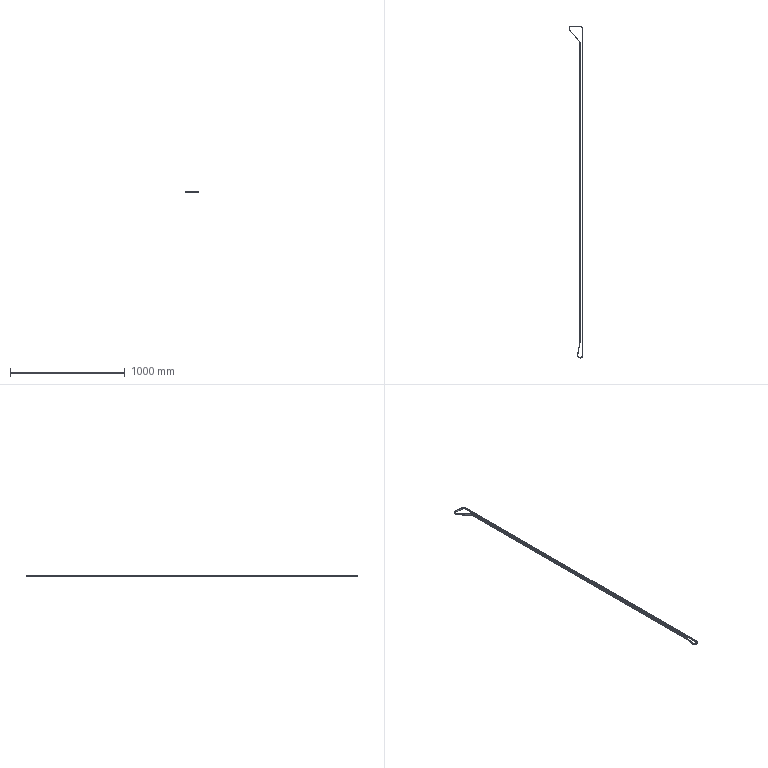Part | SolidWorks | features BaseBody 1 | 1 solid | 26 faces | box 118.8 x 2900 x 15 mm | volume 178480 mm3 | cylinder 14 | plane 12 | commonest cylinder face diameters 41.8 x5 45.8 x5 23 x2 27 x2
STEP:
#1=CARTESIAN_POINT('',(-71.857,624.869,16.));
#2=VERTEX_POINT('',#1);
#3=CARTESIAN_POINT('',(-93.9,604.,16.));
#4=VERTEX_POINT('',#3);
#5=CARTESIAN_POINT('',(-73.,604.,16.));
#6=DIRECTION('',(0.,0.,1.));
#7=DIRECTION('',(1.,0.,0.));
#8=AXIS2_PLACEMENT_3D('',#5,#6,#7);
#9=CIRCLE('',#8,20.9);
#10=EDGE_CURVE('',#2,#4,#9,.T.);
#11=ORIENTED_EDGE('',*,*,#10,.T.);
#12=CARTESIAN_POINT('',(-93.9,604.,1.));
#13=VERTEX_POINT('',#12);
#14=CARTESIAN_POINT('',(-93.9,604.,16.));
#15=DIRECTION('',(0.,0.,-1.));
#16=VECTOR('',#15,1000.);
#17=LINE('',#14,#16);
#18=EDGE_CURVE('',#4,#13,#17,.T.);
#19=ORIENTED_EDGE('',*,*,#18,.T.);
#20=CARTESIAN_POINT('',(-71.857,624.869,1.));
#21=VERTEX_POINT('',#20);
#22=CARTESIAN_POINT('',(-73.,604.,1.));
#23=DIRECTION('',(0.,0.,1.));
#24=DIRECTION('',(1.,0.,0.));
#25=AXIS2_PLACEMENT_3D('',#22,#23,#24);
#26=CIRCLE('',#25,20.9);
#27=EDGE_CURVE('',#21,#13,#26,.T.);
#28=ORIENTED_EDGE('',*,*,#27,.F.);
#29=CARTESIAN_POINT('',(-71.857,624.869,16.));
#30=DIRECTION('',(0.,0.,-1.));
#31=VECTOR('',#30,1000.);
#32=LINE('',#29,#31);
#33=EDGE_CURVE('',#2,#21,#32,.T.);
#34=ORIENTED_EDGE('',*,*,#33,.F.);
#35=EDGE_LOOP('',(#11,#19,#28,#34));
#36=FACE_OUTER_BOUND('',#35,.T.);
#37=CARTESIAN_POINT('',(-73.,604.,16.));
#38=DIRECTION('',(0.,0.,-1.));
#39=DIRECTION('',(-1.,0.,0.));
#40=AXIS2_PLACEMENT_3D('',#37,#38,#39);
#41=CYLINDRICAL_SURFACE('',#40,20.9);
#42=ADVANCED_FACE('',(#36),#41,.F.);
#43=CARTESIAN_POINT('',(-20.592,-2246.176,16.));
#44=VERTEX_POINT('',#43);
#45=CARTESIAN_POINT('',(-20.9,-2249.75,16.));
#46=VERTEX_POINT('',#45);
#47=CARTESIAN_POINT('',(-0.00005287,-2249.75,16.));
#48=DIRECTION('',(0.,0.,1.));
#49=DIRECTION('',(1.,0.,0.));
#50=AXIS2_PLACEMENT_3D('',#47,#48,#49);
#51=CIRCLE('',#50,20.9);
#52=EDGE_CURVE('',#44,#46,#51,.T.);
#53=ORIENTED_EDGE('',*,*,#52,.T.);
#54=CARTESIAN_POINT('',(-20.9,-2249.75,1.));
#55=VERTEX_POINT('',#54);
#56=CARTESIAN_POINT('',(-20.9,-2249.75,16.));
#57=DIRECTION('',(0.,0.,-1.));
#58=VECTOR('',#57,1000.);
#59=LINE('',#56,#58);
#60=EDGE_CURVE('',#46,#55,#59,.T.);
#61=ORIENTED_EDGE('',*,*,#60,.T.);
#62=CARTESIAN_POINT('',(-20.592,-2246.176,1.));
#63=VERTEX_POINT('',#62);
#64=CARTESIAN_POINT('',(-0.00005287,-2249.75,1.));
#65=DIRECTION('',(0.,0.,1.));
#66=DIRECTION('',(1.,0.,0.));
#67=AXIS2_PLACEMENT_3D('',#64,#65,#66);
#68=CIRCLE('',#67,20.9);
#69=EDGE_CURVE('',#63,#55,#68,.T.);
#70=ORIENTED_EDGE('',*,*,#69,.F.);
#71=CARTESIAN_POINT('',(-20.592,-2246.176,16.));
#72=DIRECTION('',(0.,0.,-1.));
#73=VECTOR('',#72,1000.);
#74=LINE('',#71,#73);
#75=EDGE_CURVE('',#44,#63,#74,.T.);
#76=ORIENTED_EDGE('',*,*,#75,.F.);
#77=EDGE_LOOP('',(#53,#61,#70,#76));
#78=FACE_OUTER_BOUND('',#77,.T.);
#79=CARTESIAN_POINT('',(-0.00005287,-2249.75,16.));
#80=DIRECTION('',(0.,0.,-1.));
#81=DIRECTION('',(-1.,0.,0.));
#82=AXIS2_PLACEMENT_3D('',#79,#80,#81);
#83=CYLINDRICAL_SURFACE('',#82,20.9);
#84=ADVANCED_FACE('',(#78),#83,.F.);
#85=CARTESIAN_POINT('',(-95.9,604.,16.));
#86=VERTEX_POINT('',#85);
#87=CARTESIAN_POINT('',(-90.271,588.962,16.));
#88=VERTEX_POINT('',#87);
#89=CARTESIAN_POINT('',(-73.,604.,16.));
#90=DIRECTION('',(0.,0.,1.));
#91=DIRECTION('',(-1.,0.,0.));
#92=AXIS2_PLACEMENT_3D('',#89,#90,#91);
#93=CIRCLE('',#92,22.9);
#94=EDGE_CURVE('',#86,#88,#93,.T.);
#95=ORIENTED_EDGE('',*,*,#94,.F.);
#96=CARTESIAN_POINT('',(-95.9,604.,1.));
#97=VERTEX_POINT('',#96);
#98=CARTESIAN_POINT('',(-95.9,604.,16.));
#99=DIRECTION('',(0.,0.,-1.));
#100=VECTOR('',#99,1000.);
#101=LINE('',#98,#100);
#102=EDGE_CURVE('',#86,#97,#101,.T.);
#103=ORIENTED_EDGE('',*,*,#102,.T.);
#104=CARTESIAN_POINT('',(-90.271,588.962,1.));
#105=VERTEX_POINT('',#104);
#106=CARTESIAN_POINT('',(-73.,604.,1.));
#107=DIRECTION('',(0.,0.,1.));
#108=DIRECTION('',(-1.,0.,0.));
#109=AXIS2_PLACEMENT_3D('',#106,#107,#108);
#110=CIRCLE('',#109,22.9);
#111=EDGE_CURVE('',#97,#105,#110,.T.);
#112=ORIENTED_EDGE('',*,*,#111,.T.);
#113=CARTESIAN_POINT('',(-90.271,588.962,16.));
#114=DIRECTION('',(0.,0.,-1.));
#115=VECTOR('',#114,1000.);
#116=LINE('',#113,#115);
#117=EDGE_CURVE('',#88,#105,#116,.T.);
#118=ORIENTED_EDGE('',*,*,#117,.F.);
#119=EDGE_LOOP('',(#95,#103,#112,#118));
#120=FACE_OUTER_BOUND('',#119,.T.);
#121=CARTESIAN_POINT('',(-73.,604.,16.));
#122=DIRECTION('',(0.,0.,-1.));
#123=DIRECTION('',(-1.,0.,0.));
#124=AXIS2_PLACEMENT_3D('',#121,#122,#123);
#125=CYLINDRICAL_SURFACE('',#124,22.9);
#126=ADVANCED_FACE('',(#120),#125,.T.);
#127=CARTESIAN_POINT('',(-22.9,-2249.75,16.));
#128=VERTEX_POINT('',#127);
#129=CARTESIAN_POINT('',(22.9,-2249.75,16.));
#130=VERTEX_POINT('',#129);
#131=CARTESIAN_POINT('',(-0.00005287,-2249.75,16.));
#132=DIRECTION('',(0.,0.,1.));
#133=DIRECTION('',(-1.,0.,0.));
#134=AXIS2_PLACEMENT_3D('',#131,#132,#133);
#135=CIRCLE('',#134,22.9);
#136=EDGE_CURVE('',#128,#130,#135,.T.);
#137=ORIENTED_EDGE('',*,*,#136,.F.);
#138=CARTESIAN_POINT('',(-22.9,-2249.75,1.));
#139=VERTEX_POINT('',#138);
#140=CARTESIAN_POINT('',(-22.9,-2249.75,16.));
#141=DIRECTION('',(0.,0.,-1.));
#142=VECTOR('',#141,1000.);
#143=LINE('',#140,#142);
#144=EDGE_CURVE('',#128,#139,#143,.T.);
#145=ORIENTED_EDGE('',*,*,#144,.T.);
#146=CARTESIAN_POINT('',(22.9,-2249.75,1.));
#147=VERTEX_POINT('',#146);
#148=CARTESIAN_POINT('',(-0.00005287,-2249.75,1.));
#149=DIRECTION('',(0.,0.,1.));
#150=DIRECTION('',(-1.,0.,0.));
#151=AXIS2_PLACEMENT_3D('',#148,#149,#150);
#152=CIRCLE('',#151,22.9);
#153=EDGE_CURVE('',#139,#147,#152,.T.);
#154=ORIENTED_EDGE('',*,*,#153,.T.);
#155=CARTESIAN_POINT('',(22.9,-2249.75,16.));
#156=DIRECTION('',(0.,0.,-1.));
#157=VECTOR('',#156,1000.);
#158=LINE('',#155,#157);
#159=EDGE_CURVE('',#130,#147,#158,.T.);
#160=ORIENTED_EDGE('',*,*,#159,.F.);
#161=EDGE_LOOP('',(#137,#145,#154,#160));
#162=FACE_OUTER_BOUND('',#161,.T.);
#163=CARTESIAN_POINT('',(-0.00005287,-2249.75,16.));
#164=DIRECTION('',(0.,0.,-1.));
#165=DIRECTION('',(-1.,0.,0.));
#166=AXIS2_PLACEMENT_3D('',#163,#164,#165);
#167=CYLINDRICAL_SURFACE('',#166,22.9);
#168=ADVANCED_FACE('',(#162),#167,.T.);
#169=CARTESIAN_POINT('',(-88.763,590.276,1.));
#170=VERTEX_POINT('',#169);
#171=CARTESIAN_POINT('',(-4.819,493.865,1.));
#172=VERTEX_POINT('',#171);
#173=CARTESIAN_POINT('',(-88.763,590.276,1.));
#174=DIRECTION('',(0.6567,-0.7542,0.));
#175=VECTOR('',#174,1000.);
#176=LINE('',#173,#175);
#177=EDGE_CURVE('',#170,#172,#176,.T.);
#178=ORIENTED_EDGE('',*,*,#177,.F.);
#179=CARTESIAN_POINT('',(-88.763,590.276,16.));
#180=VERTEX_POINT('',#179);
#181=CARTESIAN_POINT('',(-88.763,590.276,16.));
#182=DIRECTION('',(0.,0.,-1.));
#183=VECTOR('',#182,1000.);
#184=LINE('',#181,#183);
#185=EDGE_CURVE('',#180,#170,#184,.T.);
#186=ORIENTED_EDGE('',*,*,#185,.F.);
#187=CARTESIAN_POINT('',(-4.819,493.865,16.));
#188=VERTEX_POINT('',#187);
#189=CARTESIAN_POINT('',(-88.763,590.276,16.));
#190=DIRECTION('',(0.6567,-0.7542,0.));
#191=VECTOR('',#190,1000.);
#192=LINE('',#189,#191);
#193=EDGE_CURVE('',#180,#188,#192,.T.);
#194=ORIENTED_EDGE('',*,*,#193,.T.);
#195=CARTESIAN_POINT('',(-4.819,493.865,16.));
#196=DIRECTION('',(0.,0.,-1.));
#197=VECTOR('',#196,1000.);
#198=LINE('',#195,#197);
#199=EDGE_CURVE('',#188,#172,#198,.T.);
#200=ORIENTED_EDGE('',*,*,#199,.T.);
#201=EDGE_LOOP('',(#178,#186,#194,#200));
#202=FACE_OUTER_BOUND('',#201,.T.);
#203=CARTESIAN_POINT('',(-88.763,590.276,16.));
#204=DIRECTION('',(0.7542,0.6567,0.));
#205=DIRECTION('',(0.,0.,-1.));
#206=AXIS2_PLACEMENT_3D('',#203,#204,#205);
#207=PLANE('',#206);
#208=ADVANCED_FACE('',(#202),#207,.T.);
#209=CARTESIAN_POINT('',(1.143,620.869,1.));
#210=VERTEX_POINT('',#209);
#211=CARTESIAN_POINT('',(1.143,620.869,1.));
#212=DIRECTION('',(-0.9985,0.05471,0.));
#213=VECTOR('',#212,1000.);
#214=LINE('',#211,#213);
#215=EDGE_CURVE('',#210,#21,#214,.T.);
#216=ORIENTED_EDGE('',*,*,#215,.F.);
#217=CARTESIAN_POINT('',(1.143,620.869,16.));
#218=VERTEX_POINT('',#217);
#219=CARTESIAN_POINT('',(1.143,620.869,16.));
#220=DIRECTION('',(0.,0.,-1.));
#221=VECTOR('',#220,1000.);
#222=LINE('',#219,#221);
#223=EDGE_CURVE('',#218,#210,#222,.T.);
#224=ORIENTED_EDGE('',*,*,#223,.F.);
#225=CARTESIAN_POINT('',(1.143,620.869,16.));
#226=DIRECTION('',(-0.9985,0.05471,0.));
#227=VECTOR('',#226,1000.);
#228=LINE('',#225,#227);
#229=EDGE_CURVE('',#218,#2,#228,.T.);
#230=ORIENTED_EDGE('',*,*,#229,.T.);
#231=ORIENTED_EDGE('',*,*,#33,.T.);
#232=EDGE_LOOP('',(#216,#224,#230,#231));
#233=FACE_OUTER_BOUND('',#232,.T.);
#234=CARTESIAN_POINT('',(1.143,620.869,16.));
#235=DIRECTION('',(-0.05471,-0.9985,0.));
#236=DIRECTION('',(-0.9985,0.05471,0.));
#237=AXIS2_PLACEMENT_3D('',#234,#235,#236);
#238=PLANE('',#237);
#239=ADVANCED_FACE('',(#233),#238,.T.);
#240=CARTESIAN_POINT('',(20.9,600.,1.));
#241=VERTEX_POINT('',#240);
#242=CARTESIAN_POINT('',(-0.000000696,600.,1.));
#243=DIRECTION('',(0.,0.,1.));
#244=DIRECTION('',(1.,0.,0.));
#245=AXIS2_PLACEMENT_3D('',#242,#243,#244);
#246=CIRCLE('',#245,20.9);
#247=EDGE_CURVE('',#241,#210,#246,.T.);
#248=ORIENTED_EDGE('',*,*,#247,.F.);
#249=CARTESIAN_POINT('',(20.9,600.,16.));
#250=VERTEX_POINT('',#249);
#251=CARTESIAN_POINT('',(20.9,600.,16.));
#252=DIRECTION('',(0.,0.,-1.));
#253=VECTOR('',#252,1000.);
#254=LINE('',#251,#253);
#255=EDGE_CURVE('',#250,#241,#254,.T.);
#256=ORIENTED_EDGE('',*,*,#255,.F.);
#257=CARTESIAN_POINT('',(-0.000000696,600.,16.));
#258=DIRECTION('',(0.,0.,1.));
#259=DIRECTION('',(1.,0.,0.));
#260=AXIS2_PLACEMENT_3D('',#257,#258,#259);
#261=CIRCLE('',#260,20.9);
#262=EDGE_CURVE('',#250,#218,#261,.T.);
#263=ORIENTED_EDGE('',*,*,#262,.T.);
#264=ORIENTED_EDGE('',*,*,#223,.T.);
#265=EDGE_LOOP('',(#248,#256,#263,#264));
#266=FACE_OUTER_BOUND('',#265,.T.);
#267=CARTESIAN_POINT('',(-0.000000696,600.,16.));
#268=DIRECTION('',(0.,0.,-1.));
#269=DIRECTION('',(-1.,0.,0.));
#270=AXIS2_PLACEMENT_3D('',#267,#268,#269);
#271=CYLINDRICAL_SURFACE('',#270,20.9);
#272=ADVANCED_FACE('',(#266),#271,.F.);
#273=CARTESIAN_POINT('',(20.9,-2249.75,1.));
#274=VERTEX_POINT('',#273);
#275=CARTESIAN_POINT('',(20.9,-2249.75,1.));
#276=DIRECTION('',(0.000000018,1.,0.));
#277=VECTOR('',#276,1000.);
#278=LINE('',#275,#277);
#279=EDGE_CURVE('',#274,#241,#278,.T.);
#280=ORIENTED_EDGE('',*,*,#279,.F.);
#281=CARTESIAN_POINT('',(20.9,-2249.75,16.));
#282=VERTEX_POINT('',#281);
#283=CARTESIAN_POINT('',(20.9,-2249.75,16.));
#284=DIRECTION('',(0.,0.,-1.));
#285=VECTOR('',#284,1000.);
#286=LINE('',#283,#285);
#287=EDGE_CURVE('',#282,#274,#286,.T.);
#288=ORIENTED_EDGE('',*,*,#287,.F.);
#289=CARTESIAN_POINT('',(20.9,-2249.75,16.));
#290=DIRECTION('',(0.000000018,1.,0.));
#291=VECTOR('',#290,1000.);
#292=LINE('',#289,#291);
#293=EDGE_CURVE('',#282,#250,#292,.T.);
#294=ORIENTED_EDGE('',*,*,#293,.T.);
#295=ORIENTED_EDGE('',*,*,#255,.T.);
#296=EDGE_LOOP('',(#280,#288,#294,#295));
#297=FACE_OUTER_BOUND('',#296,.T.);
#298=CARTESIAN_POINT('',(20.9,-2249.75,16.));
#299=DIRECTION('',(-1.,0.000000018,0.));
#300=DIRECTION('',(0.,0.,1.));
#301=AXIS2_PLACEMENT_3D('',#298,#299,#300);
#302=PLANE('',#301);
#303=ADVANCED_FACE('',(#297),#302,.T.);
#304=CARTESIAN_POINT('',(-1.699,-2137.308,1.));
#305=VERTEX_POINT('',#304);
#306=CARTESIAN_POINT('',(-1.699,-2137.308,1.));
#307=DIRECTION('',(-0.171,-0.9853,0.));
#308=VECTOR('',#307,1000.);
#309=LINE('',#306,#308);
#310=EDGE_CURVE('',#305,#63,#309,.T.);
#311=ORIENTED_EDGE('',*,*,#310,.F.);
#312=CARTESIAN_POINT('',(-1.699,-2137.308,16.));
#313=VERTEX_POINT('',#312);
#314=CARTESIAN_POINT('',(-1.699,-2137.308,16.));
#315=DIRECTION('',(0.,0.,-1.));
#316=VECTOR('',#315,1000.);
#317=LINE('',#314,#316);
#318=EDGE_CURVE('',#313,#305,#317,.T.);
#319=ORIENTED_EDGE('',*,*,#318,.F.);
#320=CARTESIAN_POINT('',(-1.699,-2137.308,16.));
#321=DIRECTION('',(-0.171,-0.9853,0.));
#322=VECTOR('',#321,1000.);
#323=LINE('',#320,#322);
#324=EDGE_CURVE('',#313,#44,#323,.T.);
#325=ORIENTED_EDGE('',*,*,#324,.T.);
#326=ORIENTED_EDGE('',*,*,#75,.T.);
#327=EDGE_LOOP('',(#311,#319,#325,#326));
#328=FACE_OUTER_BOUND('',#327,.T.);
#329=CARTESIAN_POINT('',(-1.699,-2137.308,16.));
#330=DIRECTION('',(0.9853,-0.171,0.));
#331=DIRECTION('',(0.,0.,-1.));
#332=AXIS2_PLACEMENT_3D('',#329,#330,#331);
#333=PLANE('',#332);
#334=ADVANCED_FACE('',(#328),#333,.T.);
#335=CARTESIAN_POINT('',(-1.5,-2135.,1.));
#336=VERTEX_POINT('',#335);
#337=CARTESIAN_POINT('',(-15.,-2135.,1.));
#338=DIRECTION('',(0.,0.,-1.));
#339=DIRECTION('',(-1.,0.,0.));
#340=AXIS2_PLACEMENT_3D('',#337,#338,#339);
#341=CIRCLE('',#340,13.5);
#342=EDGE_CURVE('',#336,#305,#341,.T.);
#343=ORIENTED_EDGE('',*,*,#342,.F.);
#344=CARTESIAN_POINT('',(-1.5,-2135.,16.));
#345=VERTEX_POINT('',#344);
#346=CARTESIAN_POINT('',(-1.5,-2135.,16.));
#347=DIRECTION('',(0.,0.,-1.));
#348=VECTOR('',#347,1000.);
#349=LINE('',#346,#348);
#350=EDGE_CURVE('',#345,#336,#349,.T.);
#351=ORIENTED_EDGE('',*,*,#350,.F.);
#352=CARTESIAN_POINT('',(-15.,-2135.,16.));
#353=DIRECTION('',(0.,0.,-1.));
#354=DIRECTION('',(-1.,0.,0.));
#355=AXIS2_PLACEMENT_3D('',#352,#353,#354);
#356=CIRCLE('',#355,13.5);
#357=EDGE_CURVE('',#345,#313,#356,.T.);
#358=ORIENTED_EDGE('',*,*,#357,.T.);
#359=ORIENTED_EDGE('',*,*,#318,.T.);
#360=EDGE_LOOP('',(#343,#351,#358,#359));
#361=FACE_OUTER_BOUND('',#360,.T.);
#362=CARTESIAN_POINT('',(-15.,-2135.,16.));
#363=DIRECTION('',(0.,0.,-1.));
#364=DIRECTION('',(-1.,0.,0.));
#365=AXIS2_PLACEMENT_3D('',#362,#363,#364);
#366=CYLINDRICAL_SURFACE('',#365,13.5);
#367=ADVANCED_FACE('',(#361),#366,.T.);
#368=CARTESIAN_POINT('',(-1.5,485.,1.));
#369=VERTEX_POINT('',#368);
#370=CARTESIAN_POINT('',(-1.5,485.,1.));
#371=DIRECTION('',(0.,-1.,0.));
#372=VECTOR('',#371,1000.);
#373=LINE('',#370,#372);
#374=EDGE_CURVE('',#369,#336,#373,.T.);
#375=ORIENTED_EDGE('',*,*,#374,.F.);
#376=CARTESIAN_POINT('',(-1.5,485.,16.));
#377=VERTEX_POINT('',#376);
#378=CARTESIAN_POINT('',(-1.5,485.,16.));
#379=DIRECTION('',(0.,0.,-1.));
#380=VECTOR('',#379,1000.);
#381=LINE('',#378,#380);
#382=EDGE_CURVE('',#377,#369,#381,.T.);
#383=ORIENTED_EDGE('',*,*,#382,.F.);
#384=CARTESIAN_POINT('',(-1.5,485.,16.));
#385=DIRECTION('',(0.,-1.,0.));
#386=VECTOR('',#385,1000.);
#387=LINE('',#384,#386);
#388=EDGE_CURVE('',#377,#345,#387,.T.);
#389=ORIENTED_EDGE('',*,*,#388,.T.);
#390=ORIENTED_EDGE('',*,*,#350,.T.);
#391=EDGE_LOOP('',(#375,#383,#389,#390));
#392=FACE_OUTER_BOUND('',#391,.T.);
#393=CARTESIAN_POINT('',(-1.5,485.,16.));
#394=DIRECTION('',(1.,0.,0.));
#395=DIRECTION('',(0.,-1.,0.));
#396=AXIS2_PLACEMENT_3D('',#393,#394,#395);
#397=PLANE('',#396);
#398=ADVANCED_FACE('',(#392),#397,.T.);
#399=CARTESIAN_POINT('',(-15.,485.,1.));
#400=DIRECTION('',(0.,0.,-1.));
#401=DIRECTION('',(-1.,0.,0.));
#402=AXIS2_PLACEMENT_3D('',#399,#400,#401);
#403=CIRCLE('',#402,13.5);
#404=EDGE_CURVE('',#172,#369,#403,.T.);
#405=ORIENTED_EDGE('',*,*,#404,.F.);
#406=ORIENTED_EDGE('',*,*,#199,.F.);
#407=CARTESIAN_POINT('',(-15.,485.,16.));
#408=DIRECTION('',(0.,0.,-1.));
#409=DIRECTION('',(-1.,0.,0.));
#410=AXIS2_PLACEMENT_3D('',#407,#408,#409);
#411=CIRCLE('',#410,13.5);
#412=EDGE_CURVE('',#188,#377,#411,.T.);
#413=ORIENTED_EDGE('',*,*,#412,.T.);
#414=ORIENTED_EDGE('',*,*,#382,.T.);
#415=EDGE_LOOP('',(#405,#406,#413,#414));
#416=FACE_OUTER_BOUND('',#415,.T.);
#417=CARTESIAN_POINT('',(-15.,485.,16.));
#418=DIRECTION('',(0.,0.,-1.));
#419=DIRECTION('',(-1.,0.,0.));
#420=AXIS2_PLACEMENT_3D('',#417,#418,#419);
#421=CYLINDRICAL_SURFACE('',#420,13.5);
#422=ADVANCED_FACE('',(#416),#421,.T.);
#423=CARTESIAN_POINT('',(-6.327,492.552,1.));
#424=VERTEX_POINT('',#423);
#425=CARTESIAN_POINT('',(-6.327,492.552,1.));
#426=DIRECTION('',(0.6567,-0.7542,0.));
#427=VECTOR('',#426,1000.);
#428=LINE('',#425,#427);
#429=EDGE_CURVE('',#105,#424,#428,.T.);
#430=ORIENTED_EDGE('',*,*,#429,.T.);
#431=CARTESIAN_POINT('',(-6.327,492.552,16.));
#432=VERTEX_POINT('',#431);
#433=CARTESIAN_POINT('',(-6.327,492.552,16.));
#434=DIRECTION('',(0.,0.,-1.));
#435=VECTOR('',#434,1000.);
#436=LINE('',#433,#435);
#437=EDGE_CURVE('',#432,#424,#436,.T.);
#438=ORIENTED_EDGE('',*,*,#437,.F.);
#439=CARTESIAN_POINT('',(-6.327,492.552,16.));
#440=DIRECTION('',(0.6567,-0.7542,0.));
#441=VECTOR('',#440,1000.);
#442=LINE('',#439,#441);
#443=EDGE_CURVE('',#88,#432,#442,.T.);
#444=ORIENTED_EDGE('',*,*,#443,.F.);
#445=ORIENTED_EDGE('',*,*,#117,.T.);
#446=EDGE_LOOP('',(#430,#438,#444,#445));
#447=FACE_OUTER_BOUND('',#446,.T.);
#448=CARTESIAN_POINT('',(-6.327,492.552,16.));
#449=DIRECTION('',(0.7542,0.6567,0.));
#450=DIRECTION('',(0.,0.,-1.));
#451=AXIS2_PLACEMENT_3D('',#448,#449,#450);
#452=PLANE('',#451);
#453=ADVANCED_FACE('',(#447),#452,.F.);
#454=CARTESIAN_POINT('',(1.253,622.866,1.));
#455=VERTEX_POINT('',#454);
#456=CARTESIAN_POINT('',(-71.747,626.866,1.));
#457=VERTEX_POINT('',#456);
#458=CARTESIAN_POINT('',(-7.42,623.341,1.));
#459=DIRECTION('',(-0.9985,0.05471,0.));
#460=VECTOR('',#459,1000.);
#461=LINE('',#458,#460);
#462=EDGE_CURVE('',#455,#457,#461,.T.);
#463=ORIENTED_EDGE('',*,*,#462,.T.);
#464=CARTESIAN_POINT('',(-71.747,626.866,16.));
#465=VERTEX_POINT('',#464);
#466=CARTESIAN_POINT('',(-71.747,626.866,16.));
#467=DIRECTION('',(0.,0.,-1.));
#468=VECTOR('',#467,1000.);
#469=LINE('',#466,#468);
#470=EDGE_CURVE('',#465,#457,#469,.T.);
#471=ORIENTED_EDGE('',*,*,#470,.F.);
#472=CARTESIAN_POINT('',(1.253,622.866,16.));
#473=VERTEX_POINT('',#472);
#474=CARTESIAN_POINT('',(-7.42,623.341,16.));
#475=DIRECTION('',(-0.9985,0.05471,0.));
#476=VECTOR('',#475,1000.);
#477=LINE('',#474,#476);
#478=EDGE_CURVE('',#473,#465,#477,.T.);
#479=ORIENTED_EDGE('',*,*,#478,.F.);
#480=CARTESIAN_POINT('',(1.253,622.866,16.));
#481=DIRECTION('',(0.,0.,-1.));
#482=VECTOR('',#481,1000.);
#483=LINE('',#480,#482);
#484=EDGE_CURVE('',#473,#455,#483,.T.);
#485=ORIENTED_EDGE('',*,*,#484,.T.);
#486=EDGE_LOOP('',(#463,#471,#479,#485));
#487=FACE_OUTER_BOUND('',#486,.T.);
#488=CARTESIAN_POINT('',(-7.42,623.341,16.));
#489=DIRECTION('',(-0.05471,-0.9985,0.));
#490=DIRECTION('',(-0.9985,0.05471,0.));
#491=AXIS2_PLACEMENT_3D('',#488,#489,#490);
#492=PLANE('',#491);
#493=ADVANCED_FACE('',(#487),#492,.F.);
#494=CARTESIAN_POINT('',(22.9,600.,1.));
#495=VERTEX_POINT('',#494);
#496=CARTESIAN_POINT('',(-0.000000696,600.,1.));
#497=DIRECTION('',(0.,0.,1.));
#498=DIRECTION('',(-1.,0.,0.));
#499=AXIS2_PLACEMENT_3D('',#496,#497,#498);
#500=CIRCLE('',#499,22.9);
#501=EDGE_CURVE('',#495,#455,#500,.T.);
#502=ORIENTED_EDGE('',*,*,#501,.T.);
#503=ORIENTED_EDGE('',*,*,#484,.F.);
#504=CARTESIAN_POINT('',(22.9,600.,16.));
#505=VERTEX_POINT('',#504);
#506=CARTESIAN_POINT('',(-0.000000696,600.,16.));
#507=DIRECTION('',(0.,0.,1.));
#508=DIRECTION('',(-1.,0.,0.));
#509=AXIS2_PLACEMENT_3D('',#506,#507,#508);
#510=CIRCLE('',#509,22.9);
#511=EDGE_CURVE('',#505,#473,#510,.T.);
#512=ORIENTED_EDGE('',*,*,#511,.F.);
#513=CARTESIAN_POINT('',(22.9,600.,16.));
#514=DIRECTION('',(0.,0.,-1.));
#515=VECTOR('',#514,1000.);
#516=LINE('',#513,#515);
#517=EDGE_CURVE('',#505,#495,#516,.T.);
#518=ORIENTED_EDGE('',*,*,#517,.T.);
#519=EDGE_LOOP('',(#502,#503,#512,#518));
#520=FACE_OUTER_BOUND('',#519,.T.);
#521=CARTESIAN_POINT('',(-0.000000696,600.,16.));
#522=DIRECTION('',(0.,0.,-1.));
#523=DIRECTION('',(-1.,0.,0.));
#524=AXIS2_PLACEMENT_3D('',#521,#522,#523);
#525=CYLINDRICAL_SURFACE('',#524,22.9);
#526=ADVANCED_FACE('',(#520),#525,.T.);
#527=CARTESIAN_POINT('',(22.9,485.,1.));
#528=DIRECTION('',(0.000000018,1.,0.));
#529=VECTOR('',#528,1000.);
#530=LINE('',#527,#529);
#531=EDGE_CURVE('',#147,#495,#530,.T.);
#532=ORIENTED_EDGE('',*,*,#531,.T.);
#533=ORIENTED_EDGE('',*,*,#517,.F.);
#534=CARTESIAN_POINT('',(22.9,485.,16.));
#535=DIRECTION('',(0.000000018,1.,0.));
#536=VECTOR('',#535,1000.);
#537=LINE('',#534,#536);
#538=EDGE_CURVE('',#130,#505,#537,.T.);
#539=ORIENTED_EDGE('',*,*,#538,.F.);
#540=ORIENTED_EDGE('',*,*,#159,.T.);
#541=EDGE_LOOP('',(#532,#533,#539,#540));
#542=FACE_OUTER_BOUND('',#541,.T.);
#543=CARTESIAN_POINT('',(22.9,485.,16.));
#544=DIRECTION('',(-1.,0.000000018,0.));
#545=DIRECTION('',(0.,0.,1.));
#546=AXIS2_PLACEMENT_3D('',#543,#544,#545);
#547=PLANE('',#546);
#548=ADVANCED_FACE('',(#542),#547,.F.);
#549=CARTESIAN_POINT('',(-3.669,-2136.966,1.));
#550=VERTEX_POINT('',#549);
#551=CARTESIAN_POINT('',(-22.563,-2245.834,1.));
#552=VERTEX_POINT('',#551);
#553=CARTESIAN_POINT('',(437.723,406.433,1.));
#554=DIRECTION('',(-0.171,-0.9853,0.));
#555=VECTOR('',#554,1000.);
#556=LINE('',#553,#555);
#557=EDGE_CURVE('',#550,#552,#556,.T.);
#558=ORIENTED_EDGE('',*,*,#557,.T.);
#559=CARTESIAN_POINT('',(-22.563,-2245.834,16.));
#560=VERTEX_POINT('',#559);
#561=CARTESIAN_POINT('',(-22.563,-2245.834,16.));
#562=DIRECTION('',(0.,0.,-1.));
#563=VECTOR('',#562,1000.);
#564=LINE('',#561,#563);
#565=EDGE_CURVE('',#560,#552,#564,.T.);
#566=ORIENTED_EDGE('',*,*,#565,.F.);
#567=CARTESIAN_POINT('',(-3.669,-2136.966,16.));
#568=VERTEX_POINT('',#567);
#569=CARTESIAN_POINT('',(437.723,406.433,16.));
#570=DIRECTION('',(-0.171,-0.9853,0.));
#571=VECTOR('',#570,1000.);
#572=LINE('',#569,#571);
#573=EDGE_CURVE('',#568,#560,#572,.T.);
#574=ORIENTED_EDGE('',*,*,#573,.F.);
#575=CARTESIAN_POINT('',(-3.669,-2136.966,16.));
#576=DIRECTION('',(0.,0.,-1.));
#577=VECTOR('',#576,1000.);
#578=LINE('',#575,#577);
#579=EDGE_CURVE('',#568,#550,#578,.T.);
#580=ORIENTED_EDGE('',*,*,#579,.T.);
#581=EDGE_LOOP('',(#558,#566,#574,#580));
#582=FACE_OUTER_BOUND('',#581,.T.);
#583=CARTESIAN_POINT('',(437.723,406.433,16.));
#584=DIRECTION('',(0.9853,-0.171,0.));
#585=DIRECTION('',(0.,0.,-1.));
#586=AXIS2_PLACEMENT_3D('',#583,#584,#585);
#587=PLANE('',#586);
#588=ADVANCED_FACE('',(#582),#587,.F.);
#589=CARTESIAN_POINT('',(-3.5,-2135.,1.));
#590=VERTEX_POINT('',#589);
#591=CARTESIAN_POINT('',(-15.,-2135.,1.));
#592=DIRECTION('',(0.,0.,-1.));
#593=DIRECTION('',(-1.,0.,0.));
#594=AXIS2_PLACEMENT_3D('',#591,#592,#593);
#595=CIRCLE('',#594,11.5);
#596=EDGE_CURVE('',#590,#550,#595,.T.);
#597=ORIENTED_EDGE('',*,*,#596,.T.);
#598=ORIENTED_EDGE('',*,*,#579,.F.);
#599=CARTESIAN_POINT('',(-3.5,-2135.,16.));
#600=VERTEX_POINT('',#599);
#601=CARTESIAN_POINT('',(-15.,-2135.,16.));
#602=DIRECTION('',(0.,0.,-1.));
#603=DIRECTION('',(-1.,0.,0.));
#604=AXIS2_PLACEMENT_3D('',#601,#602,#603);
#605=CIRCLE('',#604,11.5);
#606=EDGE_CURVE('',#600,#568,#605,.T.);
#607=ORIENTED_EDGE('',*,*,#606,.F.);
#608=CARTESIAN_POINT('',(-3.5,-2135.,16.));
#609=DIRECTION('',(0.,0.,-1.));
#610=VECTOR('',#609,1000.);
#611=LINE('',#608,#610);
#612=EDGE_CURVE('',#600,#590,#611,.T.);
#613=ORIENTED_EDGE('',*,*,#612,.T.);
#614=EDGE_LOOP('',(#597,#598,#607,#613));
#615=FACE_OUTER_BOUND('',#614,.T.);
#616=CARTESIAN_POINT('',(-15.,-2135.,16.));
#617=DIRECTION('',(0.,0.,-1.));
#618=DIRECTION('',(-1.,0.,0.));
#619=AXIS2_PLACEMENT_3D('',#616,#617,#618);
#620=CYLINDRICAL_SURFACE('',#619,11.5);
#621=ADVANCED_FACE('',(#615),#620,.F.);
#622=CARTESIAN_POINT('',(-3.5,485.,1.));
#623=VERTEX_POINT('',#622);
#624=CARTESIAN_POINT('',(-3.5,485.,1.));
#625=DIRECTION('',(0.,-1.,0.));
#626=VECTOR('',#625,1000.);
#627=LINE('',#624,#626);
#628=EDGE_CURVE('',#623,#590,#627,.T.);
#629=ORIENTED_EDGE('',*,*,#628,.T.);
#630=ORIENTED_EDGE('',*,*,#612,.F.);
#631=CARTESIAN_POINT('',(-3.5,485.,16.));
#632=VERTEX_POINT('',#631);
#633=CARTESIAN_POINT('',(-3.5,485.,16.));
#634=DIRECTION('',(0.,-1.,0.));
#635=VECTOR('',#634,1000.);
#636=LINE('',#633,#635);
#637=EDGE_CURVE('',#632,#600,#636,.T.);
#638=ORIENTED_EDGE('',*,*,#637,.F.);
#639=CARTESIAN_POINT('',(-3.5,485.,16.));
#640=DIRECTION('',(0.,0.,-1.));
#641=VECTOR('',#640,1000.);
#642=LINE('',#639,#641);
#643=EDGE_CURVE('',#632,#623,#642,.T.);
#644=ORIENTED_EDGE('',*,*,#643,.T.);
#645=EDGE_LOOP('',(#629,#630,#638,#644));
#646=FACE_OUTER_BOUND('',#645,.T.);
#647=CARTESIAN_POINT('',(-3.5,485.,16.));
#648=DIRECTION('',(1.,0.,0.));
#649=DIRECTION('',(0.,-1.,0.));
#650=AXIS2_PLACEMENT_3D('',#647,#648,#649);
#651=PLANE('',#650);
#652=ADVANCED_FACE('',(#646),#651,.F.);
#653=CARTESIAN_POINT('',(-15.,485.,1.));
#654=DIRECTION('',(0.,0.,-1.));
#655=DIRECTION('',(-1.,0.,0.));
#656=AXIS2_PLACEMENT_3D('',#653,#654,#655);
#657=CIRCLE('',#656,11.5);
#658=EDGE_CURVE('',#424,#623,#657,.T.);
#659=ORIENTED_EDGE('',*,*,#658,.T.);
#660=ORIENTED_EDGE('',*,*,#643,.F.);
#661=CARTESIAN_POINT('',(-15.,485.,16.));
#662=DIRECTION('',(0.,0.,-1.));
#663=DIRECTION('',(-1.,0.,0.));
#664=AXIS2_PLACEMENT_3D('',#661,#662,#663);
#665=CIRCLE('',#664,11.5);
#666=EDGE_CURVE('',#432,#632,#665,.T.);
#667=ORIENTED_EDGE('',*,*,#666,.F.);
#668=ORIENTED_EDGE('',*,*,#437,.T.);
#669=EDGE_LOOP('',(#659,#660,#667,#668));
#670=FACE_OUTER_BOUND('',#669,.T.);
#671=CARTESIAN_POINT('',(-15.,485.,16.));
#672=DIRECTION('',(0.,0.,-1.));
#673=DIRECTION('',(-1.,0.,0.));
#674=AXIS2_PLACEMENT_3D('',#671,#672,#673);
#675=CYLINDRICAL_SURFACE('',#674,11.5);
#676=ADVANCED_FACE('',(#670),#675,.F.);
#677=ORIENTED_EDGE('',*,*,#177,.T.);
#678=ORIENTED_EDGE('',*,*,#404,.T.);
#679=ORIENTED_EDGE('',*,*,#374,.T.);
#680=ORIENTED_EDGE('',*,*,#342,.T.);
#681=ORIENTED_EDGE('',*,*,#310,.T.);
#682=ORIENTED_EDGE('',*,*,#69,.T.);
#683=CARTESIAN_POINT('',(-0.00005287,-2249.75,1.));
#684=DIRECTION('',(0.,0.,1.));
#685=DIRECTION('',(1.,0.,0.));
#686=AXIS2_PLACEMENT_3D('',#683,#684,#685);
#687=CIRCLE('',#686,20.9);
#688=EDGE_CURVE('',#55,#274,#687,.T.);
#689=ORIENTED_EDGE('',*,*,#688,.T.);
#690=ORIENTED_EDGE('',*,*,#279,.T.);
#691=ORIENTED_EDGE('',*,*,#247,.T.);
#692=ORIENTED_EDGE('',*,*,#215,.T.);
#693=ORIENTED_EDGE('',*,*,#27,.T.);
#694=CARTESIAN_POINT('',(-73.,604.,1.));
#695=DIRECTION('',(0.,0.,1.));
#696=DIRECTION('',(1.,0.,0.));
#697=AXIS2_PLACEMENT_3D('',#694,#695,#696);
#698=CIRCLE('',#697,20.9);
#699=EDGE_CURVE('',#13,#170,#698,.T.);
#700=ORIENTED_EDGE('',*,*,#699,.T.);
#701=EDGE_LOOP('',(#677,#678,#679,#680,#681,#682,#689,#690,#691,#692,#693,#700));
#702=FACE_BOUND('',#701,.T.);
#703=ORIENTED_EDGE('',*,*,#658,.F.);
#704=ORIENTED_EDGE('',*,*,#429,.F.);
#705=ORIENTED_EDGE('',*,*,#111,.F.);
#706=CARTESIAN_POINT('',(-73.,604.,1.));
#707=DIRECTION('',(0.,0.,1.));
#708=DIRECTION('',(-1.,0.,0.));
#709=AXIS2_PLACEMENT_3D('',#706,#707,#708);
#710=CIRCLE('',#709,22.9);
#711=EDGE_CURVE('',#457,#97,#710,.T.);
#712=ORIENTED_EDGE('',*,*,#711,.F.);
#713=ORIENTED_EDGE('',*,*,#462,.F.);
#714=ORIENTED_EDGE('',*,*,#501,.F.);
#715=ORIENTED_EDGE('',*,*,#531,.F.);
#716=ORIENTED_EDGE('',*,*,#153,.F.);
#717=CARTESIAN_POINT('',(-0.00005287,-2249.75,1.));
#718=DIRECTION('',(0.,0.,1.));
#719=DIRECTION('',(-1.,0.,0.));
#720=AXIS2_PLACEMENT_3D('',#717,#718,#719);
#721=CIRCLE('',#720,22.9);
#722=EDGE_CURVE('',#552,#139,#721,.T.);
#723=ORIENTED_EDGE('',*,*,#722,.F.);
#724=ORIENTED_EDGE('',*,*,#557,.F.);
#725=ORIENTED_EDGE('',*,*,#596,.F.);
#726=ORIENTED_EDGE('',*,*,#628,.F.);
#727=EDGE_LOOP('',(#703,#704,#705,#712,#713,#714,#715,#716,#723,#724,#725,#726));
#728=FACE_OUTER_BOUND('',#727,.T.);
#729=CARTESIAN_POINT('',(-15.,485.,1.));
#730=DIRECTION('',(0.,0.,-1.));
#731=DIRECTION('',(0.,-1.,0.));
#732=AXIS2_PLACEMENT_3D('',#729,#730,#731);
#733=PLANE('',#732);
#734=ADVANCED_FACE('',(#702,#728),#733,.T.);
#735=ORIENTED_EDGE('',*,*,#412,.F.);
#736=ORIENTED_EDGE('',*,*,#193,.F.);
#737=CARTESIAN_POINT('',(-73.,604.,16.));
#738=DIRECTION('',(0.,0.,1.));
#739=DIRECTION('',(1.,0.,0.));
#740=AXIS2_PLACEMENT_3D('',#737,#738,#739);
#741=CIRCLE('',#740,20.9);
#742=EDGE_CURVE('',#4,#180,#741,.T.);
#743=ORIENTED_EDGE('',*,*,#742,.F.);
#744=ORIENTED_EDGE('',*,*,#10,.F.);
#745=ORIENTED_EDGE('',*,*,#229,.F.);
#746=ORIENTED_EDGE('',*,*,#262,.F.);
#747=ORIENTED_EDGE('',*,*,#293,.F.);
#748=CARTESIAN_POINT('',(-0.00005287,-2249.75,16.));
#749=DIRECTION('',(0.,0.,1.));
#750=DIRECTION('',(1.,0.,0.));
#751=AXIS2_PLACEMENT_3D('',#748,#749,#750);
#752=CIRCLE('',#751,20.9);
#753=EDGE_CURVE('',#46,#282,#752,.T.);
#754=ORIENTED_EDGE('',*,*,#753,.F.);
#755=ORIENTED_EDGE('',*,*,#52,.F.);
#756=ORIENTED_EDGE('',*,*,#324,.F.);
#757=ORIENTED_EDGE('',*,*,#357,.F.);
#758=ORIENTED_EDGE('',*,*,#388,.F.);
#759=EDGE_LOOP('',(#735,#736,#743,#744,#745,#746,#747,#754,#755,#756,#757,#758));
#760=FACE_BOUND('',#759,.T.);
#761=ORIENTED_EDGE('',*,*,#666,.T.);
#762=ORIENTED_EDGE('',*,*,#637,.T.);
#763=ORIENTED_EDGE('',*,*,#606,.T.);
#764=ORIENTED_EDGE('',*,*,#573,.T.);
#765=CARTESIAN_POINT('',(-0.00005287,-2249.75,16.));
#766=DIRECTION('',(0.,0.,1.));
#767=DIRECTION('',(-1.,0.,0.));
#768=AXIS2_PLACEMENT_3D('',#765,#766,#767);
#769=CIRCLE('',#768,22.9);
#770=EDGE_CURVE('',#560,#128,#769,.T.);
#771=ORIENTED_EDGE('',*,*,#770,.T.);
#772=ORIENTED_EDGE('',*,*,#136,.T.);
#773=ORIENTED_EDGE('',*,*,#538,.T.);
#774=ORIENTED_EDGE('',*,*,#511,.T.);
#775=ORIENTED_EDGE('',*,*,#478,.T.);
#776=CARTESIAN_POINT('',(-73.,604.,16.));
#777=DIRECTION('',(0.,0.,1.));
#778=DIRECTION('',(-1.,0.,0.));
#779=AXIS2_PLACEMENT_3D('',#776,#777,#778);
#780=CIRCLE('',#779,22.9);
#781=EDGE_CURVE('',#465,#86,#780,.T.);
#782=ORIENTED_EDGE('',*,*,#781,.T.);
#783=ORIENTED_EDGE('',*,*,#94,.T.);
#784=ORIENTED_EDGE('',*,*,#443,.T.);
#785=EDGE_LOOP('',(#761,#762,#763,#764,#771,#772,#773,#774,#775,#782,#783,#784));
#786=FACE_OUTER_BOUND('',#785,.T.);
#787=CARTESIAN_POINT('',(-15.,485.,16.));
#788=DIRECTION('',(0.,0.,-1.));
#789=DIRECTION('',(0.,-1.,0.));
#790=AXIS2_PLACEMENT_3D('',#787,#788,#789);
#791=PLANE('',#790);
#792=ADVANCED_FACE('',(#760,#786),#791,.F.);
#793=ORIENTED_EDGE('',*,*,#144,.F.);
#794=ORIENTED_EDGE('',*,*,#770,.F.);
#795=ORIENTED_EDGE('',*,*,#565,.T.);
#796=ORIENTED_EDGE('',*,*,#722,.T.);
#797=EDGE_LOOP('',(#793,#794,#795,#796));
#798=FACE_OUTER_BOUND('',#797,.T.);
#799=CARTESIAN_POINT('',(-0.00005287,-2249.75,16.));
#800=DIRECTION('',(0.,0.,-1.));
#801=DIRECTION('',(-1.,0.,0.));
#802=AXIS2_PLACEMENT_3D('',#799,#800,#801);
#803=CYLINDRICAL_SURFACE('',#802,22.9);
#804=ADVANCED_FACE('',(#798),#803,.T.);
#805=ORIENTED_EDGE('',*,*,#102,.F.);
#806=ORIENTED_EDGE('',*,*,#781,.F.);
#807=ORIENTED_EDGE('',*,*,#470,.T.);
#808=ORIENTED_EDGE('',*,*,#711,.T.);
#809=EDGE_LOOP('',(#805,#806,#807,#808));
#810=FACE_OUTER_BOUND('',#809,.T.);
#811=CARTESIAN_POINT('',(-73.,604.,16.));
#812=DIRECTION('',(0.,0.,-1.));
#813=DIRECTION('',(-1.,0.,0.));
#814=AXIS2_PLACEMENT_3D('',#811,#812,#813);
#815=CYLINDRICAL_SURFACE('',#814,22.9);
#816=ADVANCED_FACE('',(#810),#815,.T.);
#817=ORIENTED_EDGE('',*,*,#60,.F.);
#818=ORIENTED_EDGE('',*,*,#753,.T.);
#819=ORIENTED_EDGE('',*,*,#287,.T.);
#820=ORIENTED_EDGE('',*,*,#688,.F.);
#821=EDGE_LOOP('',(#817,#818,#819,#820));
#822=FACE_OUTER_BOUND('',#821,.T.);
#823=CARTESIAN_POINT('',(-0.00005287,-2249.75,16.));
#824=DIRECTION('',(0.,0.,-1.));
#825=DIRECTION('',(-1.,0.,0.));
#826=AXIS2_PLACEMENT_3D('',#823,#824,#825);
#827=CYLINDRICAL_SURFACE('',#826,20.9);
#828=ADVANCED_FACE('',(#822),#827,.F.);
#829=ORIENTED_EDGE('',*,*,#18,.F.);
#830=ORIENTED_EDGE('',*,*,#742,.T.);
#831=ORIENTED_EDGE('',*,*,#185,.T.);
#832=ORIENTED_EDGE('',*,*,#699,.F.);
#833=EDGE_LOOP('',(#829,#830,#831,#832));
#834=FACE_OUTER_BOUND('',#833,.T.);
#835=CARTESIAN_POINT('',(-73.,604.,16.));
#836=DIRECTION('',(0.,0.,-1.));
#837=DIRECTION('',(-1.,0.,0.));
#838=AXIS2_PLACEMENT_3D('',#835,#836,#837);
#839=CYLINDRICAL_SURFACE('',#838,20.9);
#840=ADVANCED_FACE('',(#834),#839,.F.);
#841=CLOSED_SHELL('',(#42,#84,#126,#168,#208,#239,#272,#303,#334,#367,#398,#422,#453,#493,#526,#548,#588,#621,#652,#676,#734,#792,#804,#816,#828,#840));
#842=MANIFOLD_SOLID_BREP('',#841);
#843=CARTESIAN_POINT('',(0.,0.,0.));
#844=DIRECTION('',(0.,0.,1.));
#845=DIRECTION('',(1.,0.,0.));
#846=AXIS2_PLACEMENT_3D('',#843,#844,#845);
#847=(LENGTH_UNIT()NAMED_UNIT(*)SI_UNIT(.MILLI.,.METRE.));
#848=UNCERTAINTY_MEASURE_WITH_UNIT(LENGTH_MEASURE(0.00001),#847,'','');
#849=(NAMED_UNIT(*)PLANE_ANGLE_UNIT()SI_UNIT($,.RADIAN.));
#850=(NAMED_UNIT(*)SI_UNIT($,.STERADIAN.)SOLID_ANGLE_UNIT());
#851=(GEOMETRIC_REPRESENTATION_CONTEXT(3)GLOBAL_UNCERTAINTY_ASSIGNED_CONTEXT((#848))GLOBAL_UNIT_ASSIGNED_CONTEXT((#847,#849,#850))REPRESENTATION_CONTEXT('',''));
#852=ADVANCED_BREP_SHAPE_REPRESENTATION('',(#842,#846),#851);